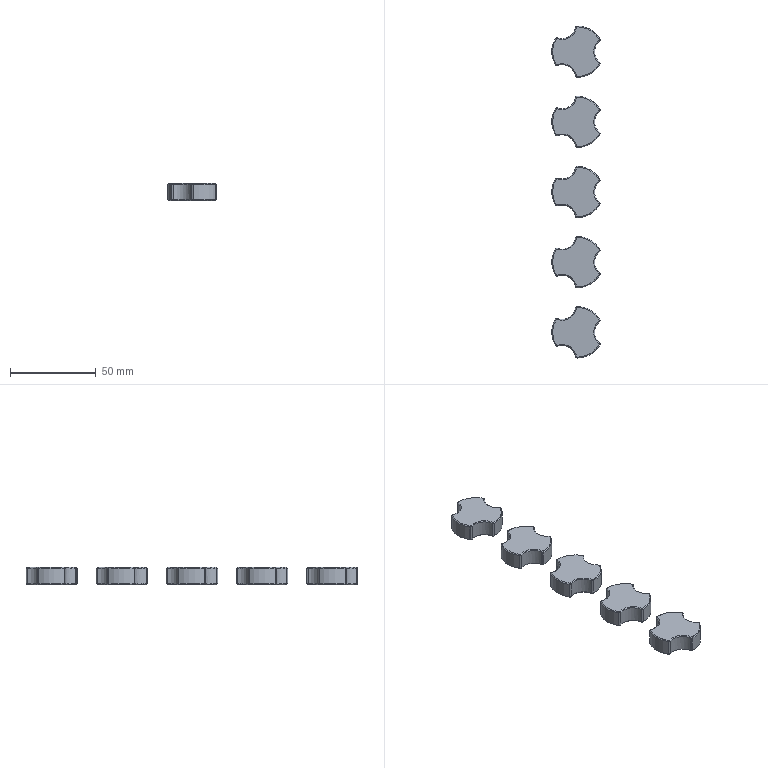Part | 5 solids | 270 faces | box 28.194 x 194 x 10 mm | volume 28053 mm3 | cone 170 | cylinder 90 | plane 10 | commonest cylinder face diameters 2 x40 16 x20 30 x20 3 x10